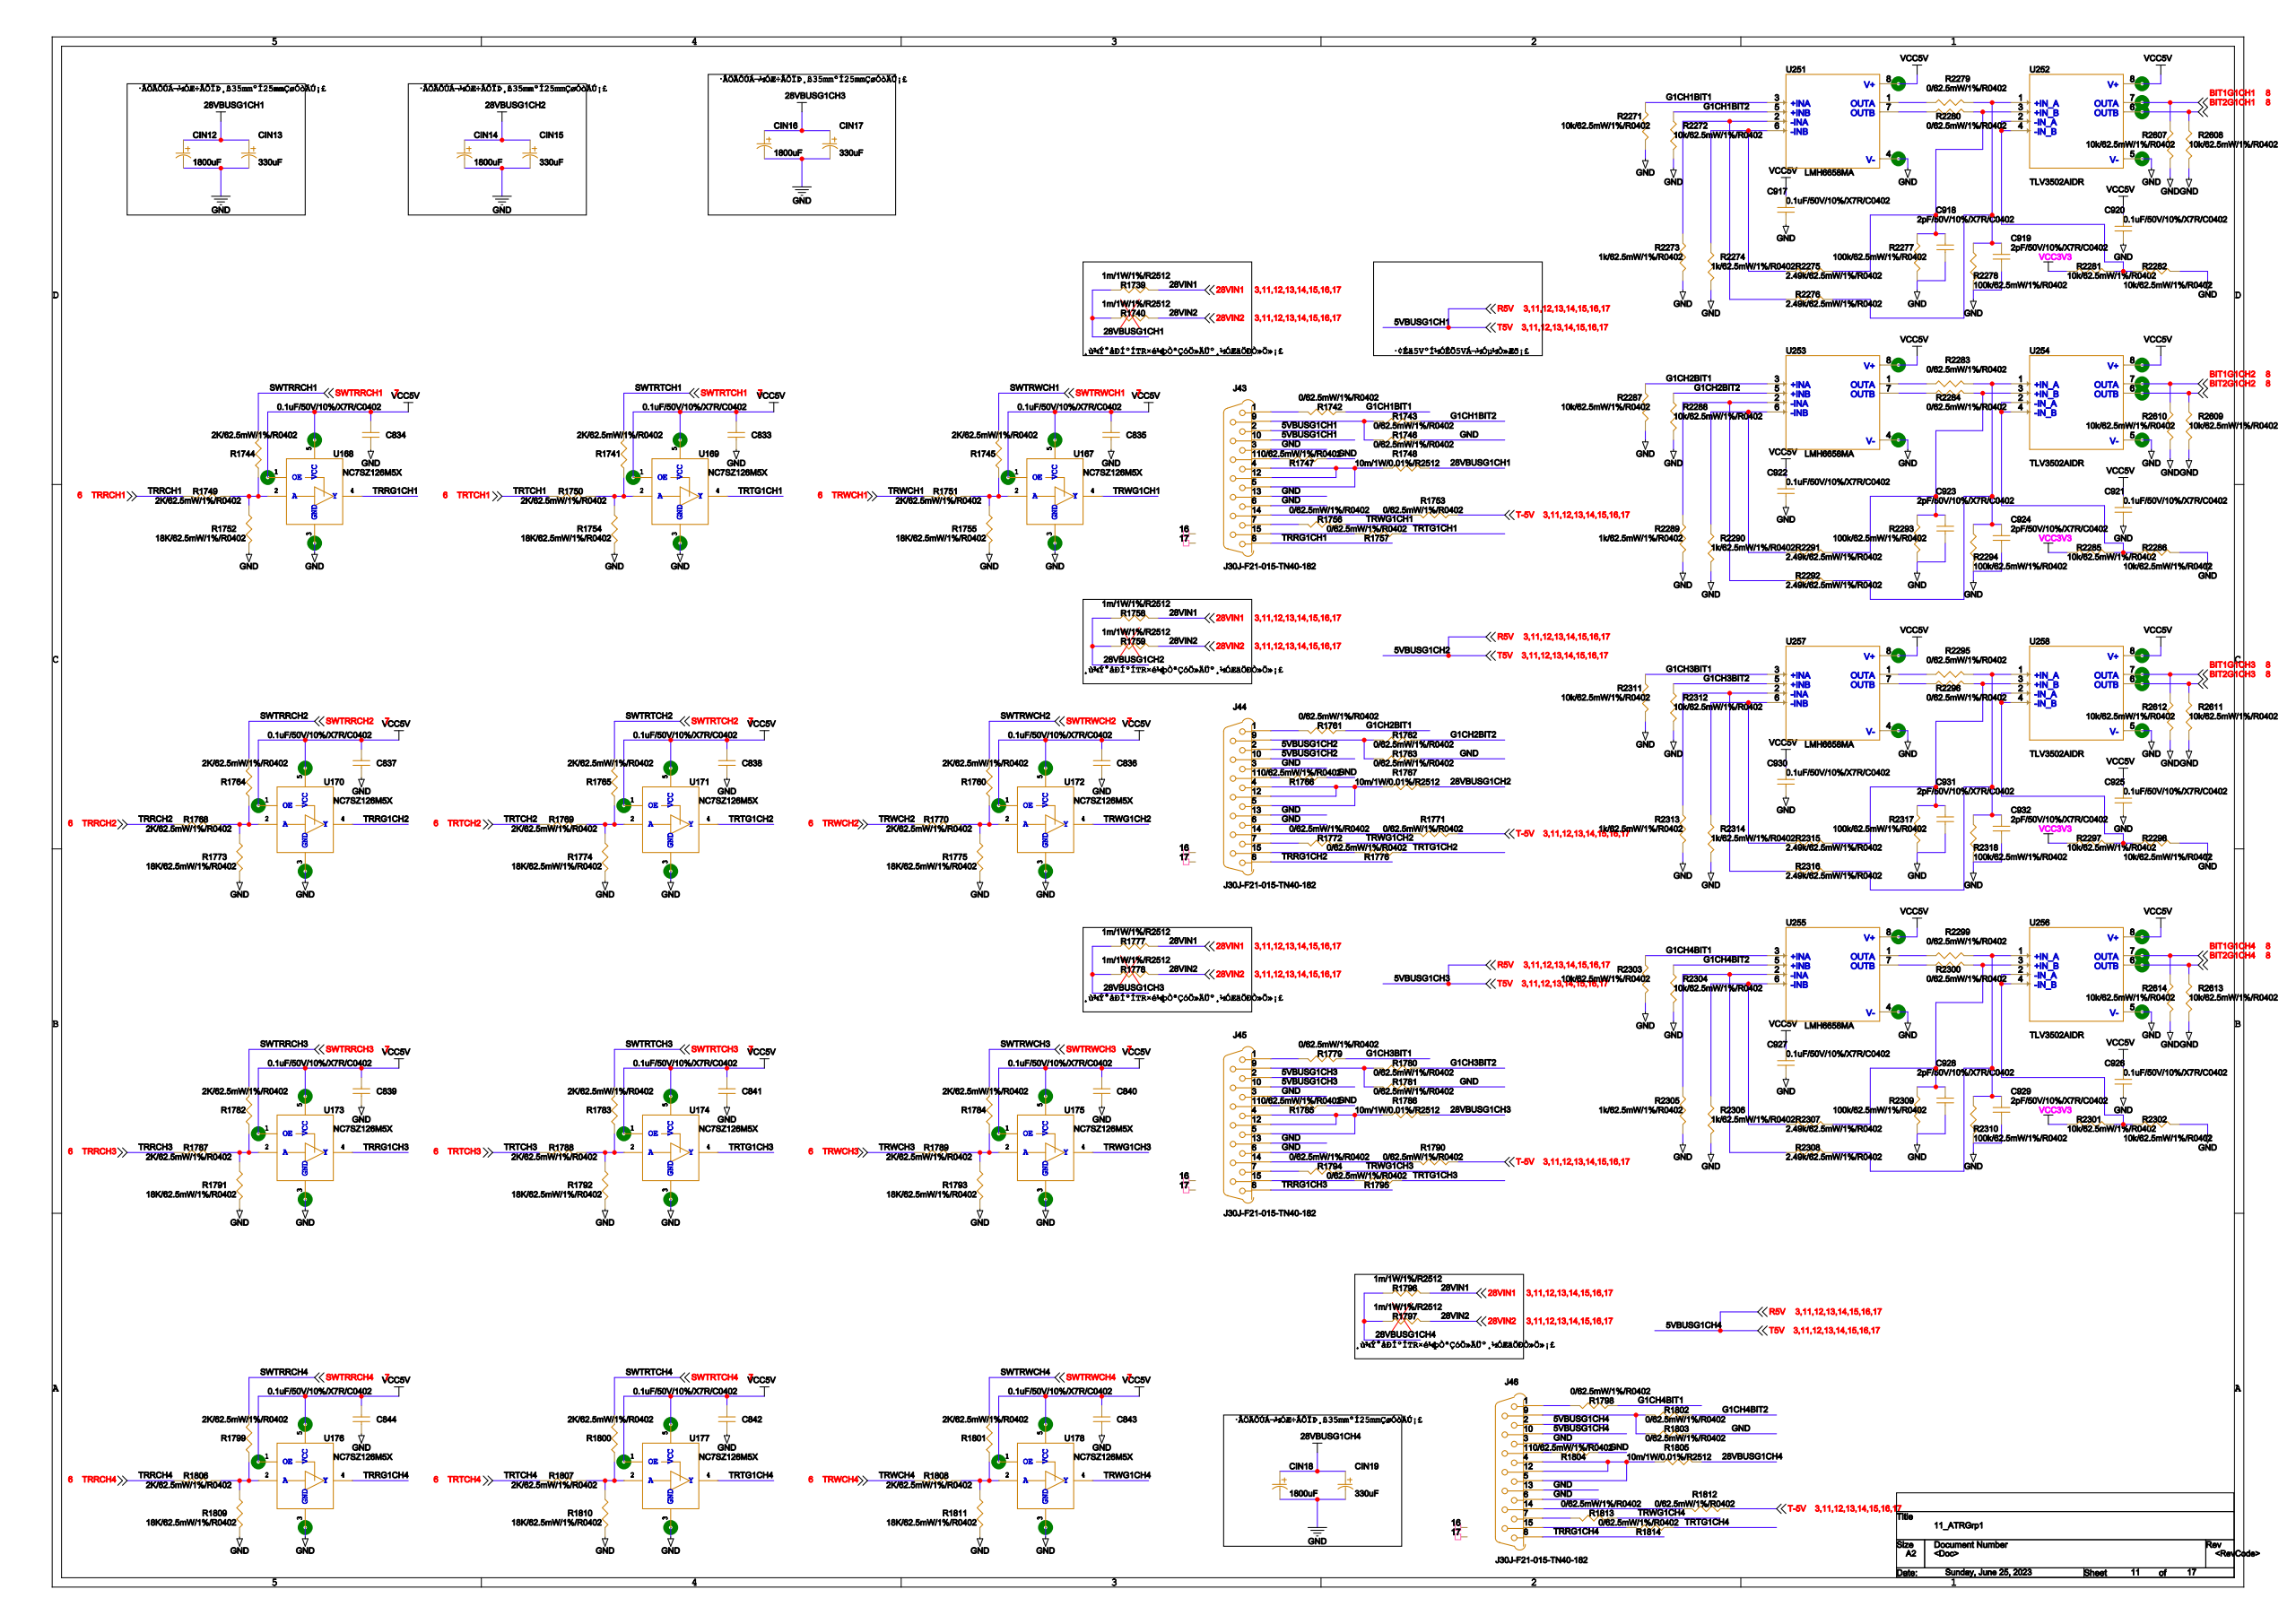Circuit board | Cadence Allegro | 2002 parts | 1538 nets | one sheet of the schematic
Parts on this sheet (reference | value | footprint):
C833 | 0.1uF/50V/10%/X7R/C0402 | 0402
C834 | 0.1uF/50V/10%/X7R/C0402 | 0402
C835 | 0.1uF/50V/10%/X7R/C0402 | 0402
C836 | 0.1uF/50V/10%/X7R/C0402 | 0402
C837 | 0.1uF/50V/10%/X7R/C0402 | 0402
C838 | 0.1uF/50V/10%/X7R/C0402 | 0402
C839 | 0.1uF/50V/10%/X7R/C0402 | 0402
C840 | 0.1uF/50V/10%/X7R/C0402 | 0402
C841 | 0.1uF/50V/10%/X7R/C0402 | 0402
C842 | 0.1uF/50V/10%/X7R/C0402 | 0402
C843 | 0.1uF/50V/10%/X7R/C0402 | 0402
C844 | 0.1uF/50V/10%/X7R/C0402 | 0402
C918 | 2pF/50V/10%/X7R/C0402 | 0402
C919 | 2pF/50V/10%/X7R/C0402 | 0402
C920 | 0.1uF/50V/10%/X7R/C0402 | 0402
C921 | 0.1uF/50V/10%/X7R/C0402 | 0402
C923 | 2pF/50V/10%/X7R/C0402 | 0402
C924 | 2pF/50V/10%/X7R/C0402 | 0402
C925 | 0.1uF/50V/10%/X7R/C0402 | 0402
C926 | 0.1uF/50V/10%/X7R/C0402 | 0402
C928 | 2pF/50V/10%/X7R/C0402 | 0402
C929 | 2pF/50V/10%/X7R/C0402 | 0402
C931 | 2pF/50V/10%/X7R/C0402 | 0402
C932 | 2pF/50V/10%/X7R/C0402 | 0402
CIN12 | ECF1HM182M27OTPO | AP-SMD_BD18-L27-W6_6-LS7_21
CIN13 | ECF1JM331G20OTPO | AP-SMD_BD10-L20-W6_6-LS7_21
CIN14 | ECF1HM182M27OTPO | AP-SMD_BD18-L27-W6_6-LS7_21
CIN15 | ECF1JM331G20OTPO | AP-SMD_BD10-L20-W6_6-LS7_21
CIN16 | ECF1HM182M27OTPO | AP-SMD_BD18-L27-W6_6-LS7_21
CIN17 | ECF1JM331G20OTPO | AP-SMD_BD10-L20-W6_6-LS7_21
CIN18 | ECF1HM182M27OTPO | AP-SMD_BD18-L27-W6_6-LS7_21
CIN19 | ECF1JM331G20OTPO | AP-SMD_BD10-L20-W6_6-LS7_21
J43 | J30J-F21-015-TN40-182 | J30J-F21-015-TN40-182
J44 | J30J-F21-015-TN40-182 | J30J-F21-015-TN40-182
J45 | J30J-F21-015-TN40-182 | J30J-F21-015-TN40-182
J46 | J30J-F21-015-TN40-182 | J30J-F21-015-TN40-182
R1739 | 1m/1W/1%/R2512 | 2512
R1740 | 1m/1W/1%/R2512 | 2512
R1741 | 2K/62.5mW/1%/R0402 | 0402
R1742 | 0/62.5mW/1%/R0402 | 0402
R1743 | 0/62.5mW/1%/R0402 | 0402
R1744 | 2K/62.5mW/1%/R0402 | 0402
R1745 | 2K/62.5mW/1%/R0402 | 0402
R1746 | 0/62.5mW/1%/R0402 | 0402
R1747 | 0/62.5mW/1%/R0402 | 0402
R1748 | 10m/1W/0.01%/R2512 | 2512
R1749 | 2K/62.5mW/1%/R0402 | 0402
R1750 | 2K/62.5mW/1%/R0402 | 0402
R1751 | 2K/62.5mW/1%/R0402 | 0402
R1752 | 18K/62.5mW/1%/R0402 | 0402
R1753 | 0/62.5mW/1%/R0402 | 0402
R1754 | 18K/62.5mW/1%/R0402 | 0402
R1755 | 18K/62.5mW/1%/R0402 | 0402
R1756 | 0/62.5mW/1%/R0402 | 0402
R1757 | 0/62.5mW/1%/R0402 | 0402
R1758 | 1m/1W/1%/R2512 | 2512
R1759 | 1m/1W/1%/R2512 | 2512
R1760 | 2K/62.5mW/1%/R0402 | 0402
R1761 | 0/62.5mW/1%/R0402 | 0402
R1762 | 0/62.5mW/1%/R0402 | 0402
R1763 | 0/62.5mW/1%/R0402 | 0402
R1764 | 2K/62.5mW/1%/R0402 | 0402
R1765 | 2K/62.5mW/1%/R0402 | 0402
R1766 | 0/62.5mW/1%/R0402 | 0402
R1767 | 10m/1W/0.01%/R2512 | 2512
R1768 | 2K/62.5mW/1%/R0402 | 0402
R1769 | 2K/62.5mW/1%/R0402 | 0402
R1770 | 2K/62.5mW/1%/R0402 | 0402
R1771 | 0/62.5mW/1%/R0402 | 0402
R1772 | 0/62.5mW/1%/R0402 | 0402
R1773 | 18K/62.5mW/1%/R0402 | 0402
R1774 | 18K/62.5mW/1%/R0402 | 0402
R1775 | 18K/62.5mW/1%/R0402 | 0402
R1776 | 0/62.5mW/1%/R0402 | 0402
R1777 | 1m/1W/1%/R2512 | 2512
R1778 | 1m/1W/1%/R2512 | 2512
R1779 | 0/62.5mW/1%/R0402 | 0402
R1780 | 0/62.5mW/1%/R0402 | 0402
R1781 | 0/62.5mW/1%/R0402 | 0402
R1782 | 2K/62.5mW/1%/R0402 | 0402
R1783 | 2K/62.5mW/1%/R0402 | 0402
R1784 | 2K/62.5mW/1%/R0402 | 0402
R1785 | 0/62.5mW/1%/R0402 | 0402
R1786 | 10m/1W/0.01%/R2512 | 2512
R1787 | 2K/62.5mW/1%/R0402 | 0402
R1788 | 2K/62.5mW/1%/R0402 | 0402
R1789 | 2K/62.5mW/1%/R0402 | 0402
R1790 | 0/62.5mW/1%/R0402 | 0402
R1791 | 18K/62.5mW/1%/R0402 | 0402
R1792 | 18K/62.5mW/1%/R0402 | 0402
R1793 | 18K/62.5mW/1%/R0402 | 0402
R1794 | 0/62.5mW/1%/R0402 | 0402
R1795 | 0/62.5mW/1%/R0402 | 0402
R1796 | 1m/1W/1%/R2512 | 2512
R1797 | 1m/1W/1%/R2512 | 2512
R1798 | 0/62.5mW/1%/R0402 | 0402
R1799 | 2K/62.5mW/1%/R0402 | 0402
R1800 | 2K/62.5mW/1%/R0402 | 0402
R1801 | 2K/62.5mW/1%/R0402 | 0402
R1802 | 0/62.5mW/1%/R0402 | 0402
R1803 | 0/62.5mW/1%/R0402 | 0402
R1804 | 0/62.5mW/1%/R0402 | 0402
R1805 | 10m/1W/0.01%/R2512 | 2512
R1806 | 2K/62.5mW/1%/R0402 | 0402
R1807 | 2K/62.5mW/1%/R0402 | 0402
R1808 | 2K/62.5mW/1%/R0402 | 0402
R1809 | 18K/62.5mW/1%/R0402 | 0402
R1810 | 18K/62.5mW/1%/R0402 | 0402
R1811 | 18K/62.5mW/1%/R0402 | 0402
R1812 | 0/62.5mW/1%/R0402 | 0402
R1813 | 0/62.5mW/1%/R0402 | 0402
R1814 | 0/62.5mW/1%/R0402 | 0402
R2271 | 10k/62.5mW/1%/R0402 | 0402
R2272 | 10k/62.5mW/1%/R0402 | 0402
R2273 | 1K/62.5mW/1%/R0402 | 0402
R2274 | 1K/62.5mW/1%/R0402 | 0402
R2276 | 2.49k/62.5mW/1%/R0402 | 0402
R2277 | 100k/62.5mW/1%/R0402 | 0402
R2278 | 100k/62.5mW/1%/R0402 | 0402
R2279 | 0/62.5mW/1%/R0402 | 0402
R2280 | 0/62.5mW/1%/R0402 | 0402
R2281 | 10k/62.5mW/1%/R0402 | 0402
R2282 | 10k/62.5mW/1%/R0402 | 0402
R2283 | 0/62.5mW/1%/R0402 | 0402
R2284 | 0/62.5mW/1%/R0402 | 0402
R2285 | 10k/62.5mW/1%/R0402 | 0402
R2286 | 10k/62.5mW/1%/R0402 | 0402
R2287 | 10k/62.5mW/1%/R0402 | 0402
R2288 | 10k/62.5mW/1%/R0402 | 0402
R2289 | 1K/62.5mW/1%/R0402 | 0402
R2290 | 1K/62.5mW/1%/R0402 | 0402
R2292 | 2.49k/62.5mW/1%/R0402 | 0402
R2293 | 100k/62.5mW/1%/R0402 | 0402
R2294 | 100k/62.5mW/1%/R0402 | 0402
R2295 | 0/62.5mW/1%/R0402 | 0402
R2296 | 0/62.5mW/1%/R0402 | 0402
R2297 | 10k/62.5mW/1%/R0402 | 0402
R2298 | 10k/62.5mW/1%/R0402 | 0402
R2299 | 0/62.5mW/1%/R0402 | 0402
R2300 | 0/62.5mW/1%/R0402 | 0402
R2301 | 10k/62.5mW/1%/R0402 | 0402
R2302 | 10k/62.5mW/1%/R0402 | 0402
R2303 | 10k/62.5mW/1%/R0402 | 0402
R2304 | 10k/62.5mW/1%/R0402 | 0402
R2305 | 1K/62.5mW/1%/R0402 | 0402
R2306 | 1K/62.5mW/1%/R0402 | 0402
R2308 | 2.49k/62.5mW/1%/R0402 | 0402
R2309 | 100k/62.5mW/1%/R0402 | 0402
R2310 | 100k/62.5mW/1%/R0402 | 0402
R2311 | 10k/62.5mW/1%/R0402 | 0402
R2312 | 10k/62.5mW/1%/R0402 | 0402
R2313 | 1K/62.5mW/1%/R0402 | 0402
R2314 | 1K/62.5mW/1%/R0402 | 0402
R2316 | 2.49k/62.5mW/1%/R0402 | 0402
R2317 | 100k/62.5mW/1%/R0402 | 0402
R2318 | 100k/62.5mW/1%/R0402 | 0402
R2607 | 10k/62.5mW/1%/R0402 | 0402
R2608 | 10k/62.5mW/1%/R0402 | 0402
R2609 | 10k/62.5mW/1%/R0402 | 0402
R2610 | 10k/62.5mW/1%/R0402 | 0402
R2611 | 10k/62.5mW/1%/R0402 | 0402
R2612 | 10k/62.5mW/1%/R0402 | 0402
R2613 | 10k/62.5mW/1%/R0402 | 0402
R2614 | 10k/62.5mW/1%/R0402 | 0402
U167 | NC7SZ126M5X | SOT-23-5
U168 | NC7SZ126M5X | SOT-23-5
U169 | NC7SZ126M5X | SOT-23-5
U170 | NC7SZ126M5X | SOT-23-5
U171 | NC7SZ126M5X | SOT-23-5
U172 | NC7SZ126M5X | SOT-23-5
U173 | NC7SZ126M5X | SOT-23-5
U174 | NC7SZ126M5X | SOT-23-5
U175 | NC7SZ126M5X | SOT-23-5
U176 | NC7SZ126M5X | SOT-23-5
U177 | NC7SZ126M5X | SOT-23-5
U178 | NC7SZ126M5X | SOT-23-5
U251 | LMH6658MA | SOIC127P599X175-8N
U253 | LMH6658MA | SOIC127P599X175-8N
U255 | LMH6658MA | SOIC127P599X175-8N
U257 | LMH6658MA | SOIC127P599X175-8N
Nets of these parts (net: part-pin ...):
3.3V: R2281-1 R2285-1 R2297-1 R2301-1
AGND: C833-2 C834-2 C835-2 C836-2 C837-2 C838-2 C839-2 C840-2 C841-2 C842-2 C843-2 C844-2 C918-2 C919-2 C920-2 C921-2 C923-2 C924-2 C925-2 C926-2 C928-2 C929-2 C931-2 C932-2 CIN12-2 CIN13-2 CIN14-2 CIN15-2 CIN16-2 CIN17-2 CIN18-2 CIN19-2 J43-3 J43-6 J43-13 J44-3 J44-6 J44-13 J45-3 J45-6 J45-13 J46-3 J46-6 J46-13 R1746-1 R1747-1 R1752-1 R1754-1 R1755-1 R1763-1 R1766-1 R1773-1 R1774-1 R1775-1 R1781-1 R1785-1 R1791-1 R1792-1 R1793-1 R1803-1 R1804-1 R1809-1 R1810-1 R1811-1 R2271-2 R2272-2 R2273-2 R2274-2 R2277-2 R2278-2 R2282-2 R2286-2 R2287-2 R2288-2 R2289-2 R2290-2 R2293-2 R2294-2 R2298-2 R2302-2 R2303-2 R2304-2 R2305-2 R2306-2 R2309-2 R2310-2 R2311-2 R2312-2 R2313-2 R2314-2 R2317-2 R2318-2 R2607-2 R2608-2 R2609-2 R2610-2 R2611-2 R2612-2 R2613-2 R2614-2 U167-3 U168-3 U169-3 U170-3 U171-3 U172-3 U173-3 U174-3 U175-3 U176-3 U177-3 U178-3 U251-4 U253-4 U255-4 U257-4
VCC5V: C833-1 C834-1 C835-1 C836-1 C837-1 C838-1 C839-1 C840-1 C841-1 C842-1 C843-1 C844-1 C920-1 C921-1 C925-1 C926-1 U167-1 U167-5 U168-1 U168-5 U169-1 U169-5 U170-1 U170-5 U171-1 U171-5 U172-1 U172-5 U173-1 U173-5 U174-1 U174-5 U175-1 U175-5 U176-1 U176-5 U177-1 U177-5 U178-1 U178-5 U251-8 U253-8 U255-8 U257-8
28VIN1: R1739-2 R1740-2 R1758-2 R1759-2 R1777-2 R1778-2 R1796-2 R1797-2
R5V: J43-2 J43-10 J44-2 J44-10 J45-2 J45-10 J46-2 J46-10
T-5V: R1753-1 R1771-1 R1790-1 R1812-1
N24388183: R2274-1 U251-6
N24388197: C918-1 R2277-1 R2280-2
N24388176: R2273-1 R2276-1 U251-2
N24388194: C919-1 R2276-2 R2278-1 R2279-2
N24389507: R2290-1 U253-6
N24389517: C923-1 R2284-2 R2293-1
N24389503: R2289-1 R2292-1 U253-2
N24389515: C924-1 R2283-2 R2292-2 R2294-1
N24391507: R2306-1 U255-6
N24391517: C928-1 R2300-2 R2309-1
N24391495: R2305-1 R2308-1 U255-2
N24391515: C929-1 R2299-2 R2308-2 R2310-1
N24391327: R2314-1 U257-6
N24391337: C931-1 R2296-2 R2317-1
N24391323: R2313-1 R2316-1 U257-2
N24391335: C932-1 R2295-2 R2316-2 R2318-1
G1CH1BIT1: R1742-1 R2271-1 U251-3
G1CH1BIT2: R1743-1 R2272-1 U251-5
N24388188: R2279-1 U251-1
N24388191: R2280-1 U251-7
G1CH2BIT1: R1761-1 R2287-1 U253-3
G1CH2BIT2: R1762-1 R2288-1 U253-5
N24389511: R2283-1 U253-1
N24389513: R2284-1 U253-7
G1CH4BIT1: R1798-1 R2303-1 U255-3
G1CH4BIT2: R1802-1 R2304-1 U255-5
N24391511: R2299-1 U255-1
N24391513: R2300-1 U255-7
G1CH3BIT1: R1779-1 R2311-1 U257-3
G1CH3BIT2: R1780-1 R2312-1 U257-5
N24391331: R2295-1 U257-1
N24391333: R2296-1 U257-7
N24388509: R2281-2 R2282-1
BIT1G1CH1: R2607-1
BIT2G1CH1: R2608-1
N24389569: R2285-2 R2286-1
BIT1G1CH2: R2610-1
BIT2G1CH2: R2609-1
N24391569: R2301-2 R2302-1
BIT1G1CH4: R2614-1
BIT2G1CH4: R2613-1
N24391389: R2297-2 R2298-1
BIT1G1CH3: R2612-1
BIT2G1CH3: R2611-1
N23704713: J43-1 R1742-2
N23704748: J43-11 R1747-2
N23704755: J43-4 J43-5 J43-12 R1748-1
N23704790: J43-14 R1753-2
N23704804: J43-15 R1757-2
N23704797: J43-7 R1756-2
TRRG1CH1: J43-8 U168-4
N23704720: J43-9 R1743-2 R1746-2
N23720843: J44-1 R1761-2
N23720856: J44-11 R1766-2
N23720858: J44-4 J44-5 J44-12 R1767-1
N23720870: J44-14 R1771-2
N23720874: J44-15 R1776-2
N23720872: J44-7 R1772-2
TRRG1CH2: J44-8 U170-4
N23720845: J44-9 R1762-2 R1763-2
N23721470: J45-1 R1779-2
N23721483: J45-11 R1785-2
N23721485: J45-4 J45-5 J45-12 R1786-1
N23721497: J45-14 R1790-2
N23721501: J45-15 R1795-2
N23721499: J45-7 R1794-2
TRRG1CH3: J45-8 U173-4
N23721472: J45-9 R1780-2 R1781-2
N23722102: J46-1 R1798-2
N23722115: J46-11 R1804-2
N23722117: J46-4 J46-5 J46-12 R1805-1
N23722129: J46-14 R1812-2
N23722133: J46-15 R1814-2
N23722131: J46-7 R1813-2
TRRG1CH4: J46-8 U176-4
N23722104: J46-9 R1802-2 R1803-2
28VBUSG1CH1: CIN12-1 CIN13-1 R1739-1 R1740-1 R1748-2
28VBUSG1CH2: CIN14-1 CIN15-1 R1758-1 R1759-1 R1767-2
28VBUSG1CH3: CIN16-1 CIN17-1 R1777-1 R1778-1 R1786-2
28VBUSG1CH4: CIN18-1 CIN19-1 R1796-1 R1797-1 R1805-2
SWTRTCH1: R1741-1
N23998857: R1741-2 R1750-2 R1754-2 U169-2
SWTRRCH1: R1744-1
N23980235: R1744-2 R1749-2 R1752-2 U168-2
SWTRWCH1: R1745-1
N23999942: R1745-2 R1751-2 R1755-2 U167-2
TRRCH1: R1749-1
TRTCH1: R1750-1
TRWCH1: R1751-1
SWTRWCH2: R1760-1
N24000060: R1760-2 R1770-2 R1775-2 U172-2
SWTRRCH2: R1764-1
N23995239: R1764-2 R1768-2 R1773-2 U170-2
SWTRTCH2: R1765-1
N23998975: R1765-2 R1769-2 R1774-2 U171-2
TRRCH2: R1768-1
TRTCH2: R1769-1
TRWCH2: R1770-1
SWTRRCH3: R1782-1
N23995539: R1782-2 R1787-2 R1791-2 U173-2
SWTRTCH3: R1783-1
N23999101: R1783-2 R1788-2 R1792-2 U174-2
SWTRWCH3: R1784-1
N24000186: R1784-2 R1789-2 R1793-2 U175-2
TRRCH3: R1787-1
TRTCH3: R1788-1
TRWCH3: R1789-1
SWTRRCH4: R1799-1
N23995853: R1799-2 R1806-2 R1809-2 U176-2
SWTRTCH4: R1800-1
N23999219: R1800-2 R1807-2 R1810-2 U177-2
SWTRWCH4: R1801-1
N24000304: R1801-2 R1808-2 R1811-2 U178-2
TRRCH4: R1806-1
TRTCH4: R1807-1
TRWCH4: R1808-1
TRWG1CH1: R1756-1 U167-4
TRTG1CH1: R1757-1 U169-4
TRTG1CH2: R1776-1 U171-4
TRWG1CH2: R1772-1 U172-4
TRTG1CH3: R1795-1 U174-4
TRWG1CH3: R1794-1 U175-4
TRTG1CH4: R1814-1 U177-4
TRWG1CH4: R1813-1 U178-4